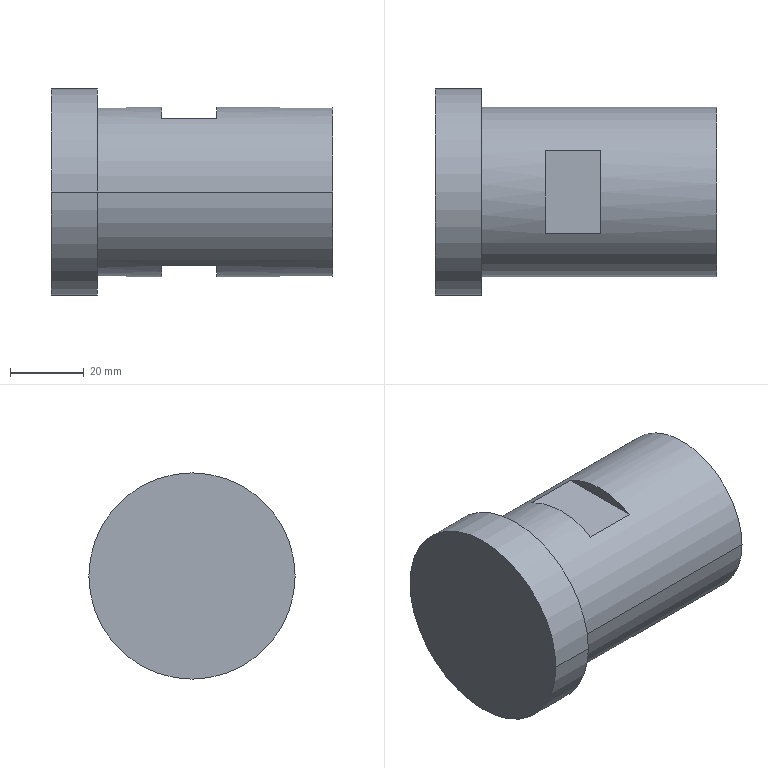Part | STEP file | DAU NOI BUA GIUA | 1 solid | 19 faces | box 76.5 x 56 x 56 mm | volume 107628 mm3 | plane 11 | cylinder 8 | commonest cylinder face diameters 33 x2 36 x2 46 x2 56 x2
STEP:
#1=CARTESIAN_POINT('',(0.,0.,0.));
#2=DIRECTION('',(0.,0.,1.));
#3=DIRECTION('',(1.,0.,0.));
#4=AXIS2_PLACEMENT_3D('',#1,#2,#3);
#5=CARTESIAN_POINT('',(45.,11.358,20.));
#6=VERTEX_POINT('',#5);
#7=CARTESIAN_POINT('',(45.,-11.358,20.));
#8=VERTEX_POINT('',#7);
#9=CARTESIAN_POINT('',(45.,0.,0.));
#10=DIRECTION('',(1.,0.,0.));
#11=DIRECTION('',(0.,1.,0.));
#12=AXIS2_PLACEMENT_3D('',#9,#10,#11);
#13=CIRCLE('',#12,23.);
#14=CARTESIAN_POINT('',(47.5,0.,0.));
#15=DIRECTION('',(1.,0.,0.));
#16=DIRECTION('',(0.,1.,0.));
#17=AXIS2_PLACEMENT_3D('',#14,#15,#16);
#18=CYLINDRICAL_SURFACE('',#17,23.);
#19=CARTESIAN_POINT('',(0.,-2.5));
#20=DIRECTION('',(1.,0.));
#21=VECTOR('',#20,1.);
#22=LINE('',#19,#21);
#23=(GEOMETRIC_REPRESENTATION_CONTEXT(2)PARAMETRIC_REPRESENTATION_CONTEXT()REPRESENTATION_CONTEXT('',''));
#24=DEFINITIONAL_REPRESENTATION('',(#22),#23);
#25=PCURVE('',#18,#24);
#26=CARTESIAN_POINT('',(45.,0.,20.));
#27=DIRECTION('',(1.,0.,0.));
#28=DIRECTION('',(0.,0.,-1.));
#29=AXIS2_PLACEMENT_3D('',#26,#27,#28);
#30=PLANE('',#29);
#31=CARTESIAN_POINT('',(20.,0.));
#32=DIRECTION('',(0.,1.));
#33=AXIS2_PLACEMENT_2D('',#31,#32);
#34=CIRCLE('',#33,23.);
#35=(GEOMETRIC_REPRESENTATION_CONTEXT(2)PARAMETRIC_REPRESENTATION_CONTEXT()REPRESENTATION_CONTEXT('',''));
#36=DEFINITIONAL_REPRESENTATION('',(#34),#35);
#37=PCURVE('',#30,#36);
#38=SURFACE_CURVE('',#13,(#25,#37),.PCURVE_S1.);
#39=EDGE_CURVE('',#6,#8,#38,.T.);
#40=ORIENTED_EDGE('',*,*,#39,.T.);
#41=CARTESIAN_POINT('',(30.,-11.358,20.));
#42=VERTEX_POINT('',#41);
#43=CARTESIAN_POINT('',(47.5,-11.358,20.));
#44=DIRECTION('',(-1.,0.,0.));
#45=VECTOR('',#44,1.);
#46=LINE('',#43,#45);
#47=CARTESIAN_POINT('',(2.087,0.));
#48=DIRECTION('',(0.,-1.));
#49=VECTOR('',#48,1.);
#50=LINE('',#47,#49);
#51=(GEOMETRIC_REPRESENTATION_CONTEXT(2)PARAMETRIC_REPRESENTATION_CONTEXT()REPRESENTATION_CONTEXT('',''));
#52=DEFINITIONAL_REPRESENTATION('',(#50),#51);
#53=PCURVE('',#18,#52);
#54=CARTESIAN_POINT('',(30.,0.,20.));
#55=DIRECTION('',(0.,0.,-1.));
#56=DIRECTION('',(-1.,0.,0.));
#57=AXIS2_PLACEMENT_3D('',#54,#55,#56);
#58=PLANE('',#57);
#59=CARTESIAN_POINT('',(-17.5,-11.358));
#60=DIRECTION('',(1.,0.));
#61=VECTOR('',#60,1.);
#62=LINE('',#59,#61);
#63=(GEOMETRIC_REPRESENTATION_CONTEXT(2)PARAMETRIC_REPRESENTATION_CONTEXT()REPRESENTATION_CONTEXT('',''));
#64=DEFINITIONAL_REPRESENTATION('',(#62),#63);
#65=PCURVE('',#58,#64);
#66=SURFACE_CURVE('',#46,(#53,#65),.PCURVE_S1.);
#67=EDGE_CURVE('',#8,#42,#66,.T.);
#68=ORIENTED_EDGE('',*,*,#67,.T.);
#69=CARTESIAN_POINT('',(30.,11.358,20.));
#70=VERTEX_POINT('',#69);
#71=CARTESIAN_POINT('',(30.,0.,0.));
#72=DIRECTION('',(-1.,0.,0.));
#73=DIRECTION('',(0.,1.,0.));
#74=AXIS2_PLACEMENT_3D('',#71,#72,#73);
#75=CIRCLE('',#74,23.);
#76=CARTESIAN_POINT('',(6.283,-17.5));
#77=DIRECTION('',(-1.,0.));
#78=VECTOR('',#77,1.);
#79=LINE('',#76,#78);
#80=(GEOMETRIC_REPRESENTATION_CONTEXT(2)PARAMETRIC_REPRESENTATION_CONTEXT()REPRESENTATION_CONTEXT('',''));
#81=DEFINITIONAL_REPRESENTATION('',(#79),#80);
#82=PCURVE('',#18,#81);
#83=CARTESIAN_POINT('',(30.,0.,30.));
#84=DIRECTION('',(-1.,0.,0.));
#85=DIRECTION('',(0.,0.,1.));
#86=AXIS2_PLACEMENT_3D('',#83,#84,#85);
#87=PLANE('',#86);
#88=CARTESIAN_POINT('',(-30.,0.));
#89=DIRECTION('',(0.,1.));
#90=AXIS2_PLACEMENT_2D('',#88,#89);
#91=CIRCLE('',#90,23.);
#92=(GEOMETRIC_REPRESENTATION_CONTEXT(2)PARAMETRIC_REPRESENTATION_CONTEXT()REPRESENTATION_CONTEXT('',''));
#93=DEFINITIONAL_REPRESENTATION('',(#91),#92);
#94=PCURVE('',#87,#93);
#95=SURFACE_CURVE('',#75,(#82,#94),.PCURVE_S1.);
#96=EDGE_CURVE('',#42,#70,#95,.T.);
#97=ORIENTED_EDGE('',*,*,#96,.T.);
#98=CARTESIAN_POINT('',(47.5,11.358,20.));
#99=DIRECTION('',(1.,0.,0.));
#100=VECTOR('',#99,1.);
#101=LINE('',#98,#100);
#102=CARTESIAN_POINT('',(1.054,0.));
#103=DIRECTION('',(0.,1.));
#104=VECTOR('',#103,1.);
#105=LINE('',#102,#104);
#106=(GEOMETRIC_REPRESENTATION_CONTEXT(2)PARAMETRIC_REPRESENTATION_CONTEXT()REPRESENTATION_CONTEXT('',''));
#107=DEFINITIONAL_REPRESENTATION('',(#105),#106);
#108=PCURVE('',#18,#107);
#109=CARTESIAN_POINT('',(-17.5,11.358));
#110=DIRECTION('',(-1.,0.));
#111=VECTOR('',#110,1.);
#112=LINE('',#109,#111);
#113=(GEOMETRIC_REPRESENTATION_CONTEXT(2)PARAMETRIC_REPRESENTATION_CONTEXT()REPRESENTATION_CONTEXT('',''));
#114=DEFINITIONAL_REPRESENTATION('',(#112),#113);
#115=PCURVE('',#58,#114);
#116=SURFACE_CURVE('',#101,(#108,#115),.PCURVE_S1.);
#117=EDGE_CURVE('',#70,#6,#116,.T.);
#118=ORIENTED_EDGE('',*,*,#117,.T.);
#119=EDGE_LOOP('',(#40,#68,#97,#118));
#120=FACE_BOUND('',#119,.T.);
#121=CARTESIAN_POINT('',(12.5,23.,0.));
#122=VERTEX_POINT('',#121);
#123=CARTESIAN_POINT('',(12.5,-23.,0.));
#124=VERTEX_POINT('',#123);
#125=CARTESIAN_POINT('',(12.5,0.,0.));
#126=DIRECTION('',(1.,0.,0.));
#127=DIRECTION('',(0.,1.,0.));
#128=AXIS2_PLACEMENT_3D('',#125,#126,#127);
#129=CIRCLE('',#128,23.);
#130=CARTESIAN_POINT('',(0.,-35.));
#131=DIRECTION('',(1.,0.));
#132=VECTOR('',#131,1.);
#133=LINE('',#130,#132);
#134=(GEOMETRIC_REPRESENTATION_CONTEXT(2)PARAMETRIC_REPRESENTATION_CONTEXT()REPRESENTATION_CONTEXT('',''));
#135=DEFINITIONAL_REPRESENTATION('',(#133),#134);
#136=PCURVE('',#18,#135);
#137=CARTESIAN_POINT('',(12.5,25.5,0.));
#138=DIRECTION('',(1.,0.,0.));
#139=DIRECTION('',(0.,0.,-1.));
#140=AXIS2_PLACEMENT_3D('',#137,#138,#139);
#141=PLANE('',#140);
#142=CARTESIAN_POINT('',(0.,-25.5));
#143=DIRECTION('',(0.,1.));
#144=AXIS2_PLACEMENT_2D('',#142,#143);
#145=CIRCLE('',#144,23.);
#146=(GEOMETRIC_REPRESENTATION_CONTEXT(2)PARAMETRIC_REPRESENTATION_CONTEXT()REPRESENTATION_CONTEXT('',''));
#147=DEFINITIONAL_REPRESENTATION('',(#145),#146);
#148=PCURVE('',#141,#147);
#149=SURFACE_CURVE('',#129,(#136,#148),.PCURVE_S1.);
#150=EDGE_CURVE('',#122,#124,#149,.T.);
#151=ORIENTED_EDGE('',*,*,#150,.T.);
#152=CARTESIAN_POINT('',(76.5,-23.,0.));
#153=VERTEX_POINT('',#152);
#154=CARTESIAN_POINT('',(47.5,-23.,0.));
#155=DIRECTION('',(1.,0.,0.));
#156=VECTOR('',#155,1.);
#157=LINE('',#154,#156);
#158=CARTESIAN_POINT('',(3.142,0.));
#159=DIRECTION('',(0.,1.));
#160=VECTOR('',#159,1.);
#161=LINE('',#158,#160);
#162=(GEOMETRIC_REPRESENTATION_CONTEXT(2)PARAMETRIC_REPRESENTATION_CONTEXT()REPRESENTATION_CONTEXT('',''));
#163=DEFINITIONAL_REPRESENTATION('',(#161),#162);
#164=PCURVE('',#18,#163);
#165=CARTESIAN_POINT('',(47.5,0.,0.));
#166=DIRECTION('',(1.,0.,0.));
#167=DIRECTION('',(0.,1.,0.));
#168=AXIS2_PLACEMENT_3D('',#165,#166,#167);
#169=CYLINDRICAL_SURFACE('',#168,23.);
#170=CARTESIAN_POINT('',(3.142,0.));
#171=DIRECTION('',(0.,1.));
#172=VECTOR('',#171,1.);
#173=LINE('',#170,#172);
#174=(GEOMETRIC_REPRESENTATION_CONTEXT(2)PARAMETRIC_REPRESENTATION_CONTEXT()REPRESENTATION_CONTEXT('',''));
#175=DEFINITIONAL_REPRESENTATION('',(#173),#174);
#176=PCURVE('',#169,#175);
#177=SURFACE_CURVE('',#157,(#164,#176),.PCURVE_S1.);
#178=EDGE_CURVE('',#124,#153,#177,.T.);
#179=ORIENTED_EDGE('',*,*,#178,.T.);
#180=CARTESIAN_POINT('',(76.5,23.,0.));
#181=VERTEX_POINT('',#180);
#182=CARTESIAN_POINT('',(76.5,0.,0.));
#183=DIRECTION('',(-1.,0.,0.));
#184=DIRECTION('',(0.,1.,0.));
#185=AXIS2_PLACEMENT_3D('',#182,#183,#184);
#186=CIRCLE('',#185,23.);
#187=CARTESIAN_POINT('',(6.283,29.));
#188=DIRECTION('',(-1.,0.));
#189=VECTOR('',#188,1.);
#190=LINE('',#187,#189);
#191=(GEOMETRIC_REPRESENTATION_CONTEXT(2)PARAMETRIC_REPRESENTATION_CONTEXT()REPRESENTATION_CONTEXT('',''));
#192=DEFINITIONAL_REPRESENTATION('',(#190),#191);
#193=PCURVE('',#18,#192);
#194=CARTESIAN_POINT('',(76.5,0.,0.));
#195=DIRECTION('',(-1.,0.,0.));
#196=DIRECTION('',(0.,0.,1.));
#197=AXIS2_PLACEMENT_3D('',#194,#195,#196);
#198=PLANE('',#197);
#199=CARTESIAN_POINT('',(0.,0.));
#200=DIRECTION('',(0.,1.));
#201=AXIS2_PLACEMENT_2D('',#199,#200);
#202=CIRCLE('',#201,23.);
#203=(GEOMETRIC_REPRESENTATION_CONTEXT(2)PARAMETRIC_REPRESENTATION_CONTEXT()REPRESENTATION_CONTEXT('',''));
#204=DEFINITIONAL_REPRESENTATION('',(#202),#203);
#205=PCURVE('',#198,#204);
#206=SURFACE_CURVE('',#186,(#193,#205),.PCURVE_S1.);
#207=EDGE_CURVE('',#153,#181,#206,.T.);
#208=ORIENTED_EDGE('',*,*,#207,.T.);
#209=CARTESIAN_POINT('',(47.5,23.,0.));
#210=DIRECTION('',(1.,0.,0.));
#211=VECTOR('',#210,1.);
#212=LINE('',#209,#211);
#213=CARTESIAN_POINT('',(0.,0.));
#214=DIRECTION('',(0.,1.));
#215=VECTOR('',#214,1.);
#216=LINE('',#213,#215);
#217=(GEOMETRIC_REPRESENTATION_CONTEXT(2)PARAMETRIC_REPRESENTATION_CONTEXT()REPRESENTATION_CONTEXT('',''));
#218=DEFINITIONAL_REPRESENTATION('',(#216),#217);
#219=PCURVE('',#18,#218);
#220=CARTESIAN_POINT('',(6.283,0.));
#221=DIRECTION('',(0.,1.));
#222=VECTOR('',#221,1.);
#223=LINE('',#220,#222);
#224=(GEOMETRIC_REPRESENTATION_CONTEXT(2)PARAMETRIC_REPRESENTATION_CONTEXT()REPRESENTATION_CONTEXT('',''));
#225=DEFINITIONAL_REPRESENTATION('',(#223),#224);
#226=PCURVE('',#169,#225);
#227=SURFACE_CURVE('',#212,(#219,#226),.PCURVE_S1.);
#228=EDGE_CURVE('',#122,#181,#227,.T.);
#229=ORIENTED_EDGE('',*,*,#228,.F.);
#230=EDGE_LOOP('',(#151,#179,#208,#229));
#231=FACE_BOUND('',#230,.T.);
#232=ADVANCED_FACE('',(#120,#231),#18,.T.);
#233=CARTESIAN_POINT('',(0.,28.,0.));
#234=VERTEX_POINT('',#233);
#235=CARTESIAN_POINT('',(0.,-28.,0.));
#236=VERTEX_POINT('',#235);
#237=CARTESIAN_POINT('',(0.,0.,0.));
#238=DIRECTION('',(1.,0.,0.));
#239=DIRECTION('',(0.,1.,0.));
#240=AXIS2_PLACEMENT_3D('',#237,#238,#239);
#241=CIRCLE('',#240,28.);
#242=CARTESIAN_POINT('',(6.25,0.,0.));
#243=DIRECTION('',(1.,0.,0.));
#244=DIRECTION('',(0.,1.,0.));
#245=AXIS2_PLACEMENT_3D('',#242,#243,#244);
#246=CYLINDRICAL_SURFACE('',#245,28.);
#247=CARTESIAN_POINT('',(0.,-6.25));
#248=DIRECTION('',(1.,0.));
#249=VECTOR('',#248,1.);
#250=LINE('',#247,#249);
#251=(GEOMETRIC_REPRESENTATION_CONTEXT(2)PARAMETRIC_REPRESENTATION_CONTEXT()REPRESENTATION_CONTEXT('',''));
#252=DEFINITIONAL_REPRESENTATION('',(#250),#251);
#253=PCURVE('',#246,#252);
#254=CARTESIAN_POINT('',(0.,14.,0.));
#255=DIRECTION('',(-1.,0.,0.));
#256=DIRECTION('',(0.,0.,1.));
#257=AXIS2_PLACEMENT_3D('',#254,#255,#256);
#258=PLANE('',#257);
#259=CARTESIAN_POINT('',(0.,14.));
#260=CARTESIAN_POINT('',(48.497,14.));
#261=CARTESIAN_POINT('',(24.249,-28.));
#262=CARTESIAN_POINT('',(0.,-70.));
#263=CARTESIAN_POINT('',(-24.249,-28.));
#264=CARTESIAN_POINT('',(-48.497,14.));
#265=CARTESIAN_POINT('',(0.,14.));
#266=(BOUNDED_CURVE()B_SPLINE_CURVE(2,(#259,#260,#261,#262,#263,#264,#265),.UNSPECIFIED.,.T.,.F.)B_SPLINE_CURVE_WITH_KNOTS((1,2,2,2,2,1),(-2.094,0.,2.094,4.189,6.283,8.378),.UNSPECIFIED.)CURVE()GEOMETRIC_REPRESENTATION_ITEM()RATIONAL_B_SPLINE_CURVE((1.,0.5,1.,0.5,1.,0.5,1.))REPRESENTATION_ITEM(''));
#267=(GEOMETRIC_REPRESENTATION_CONTEXT(2)PARAMETRIC_REPRESENTATION_CONTEXT()REPRESENTATION_CONTEXT('',''));
#268=DEFINITIONAL_REPRESENTATION('',(#266),#267);
#269=PCURVE('',#258,#268);
#270=SURFACE_CURVE('',#241,(#253,#269),.PCURVE_S1.);
#271=EDGE_CURVE('',#234,#236,#270,.T.);
#272=ORIENTED_EDGE('',*,*,#271,.T.);
#273=CARTESIAN_POINT('',(12.5,-28.,0.));
#274=VERTEX_POINT('',#273);
#275=CARTESIAN_POINT('',(6.25,-28.,0.));
#276=DIRECTION('',(1.,0.,0.));
#277=VECTOR('',#276,1.);
#278=LINE('',#275,#277);
#279=CARTESIAN_POINT('',(3.142,0.));
#280=DIRECTION('',(0.,1.));
#281=VECTOR('',#280,1.);
#282=LINE('',#279,#281);
#283=(GEOMETRIC_REPRESENTATION_CONTEXT(2)PARAMETRIC_REPRESENTATION_CONTEXT()REPRESENTATION_CONTEXT('',''));
#284=DEFINITIONAL_REPRESENTATION('',(#282),#283);
#285=PCURVE('',#246,#284);
#286=CARTESIAN_POINT('',(6.25,0.,0.));
#287=DIRECTION('',(1.,0.,0.));
#288=DIRECTION('',(0.,1.,0.));
#289=AXIS2_PLACEMENT_3D('',#286,#287,#288);
#290=CYLINDRICAL_SURFACE('',#289,28.);
#291=CARTESIAN_POINT('',(3.142,0.));
#292=DIRECTION('',(0.,1.));
#293=VECTOR('',#292,1.);
#294=LINE('',#291,#293);
#295=(GEOMETRIC_REPRESENTATION_CONTEXT(2)PARAMETRIC_REPRESENTATION_CONTEXT()REPRESENTATION_CONTEXT('',''));
#296=DEFINITIONAL_REPRESENTATION('',(#294),#295);
#297=PCURVE('',#290,#296);
#298=SURFACE_CURVE('',#278,(#285,#297),.PCURVE_S1.);
#299=EDGE_CURVE('',#236,#274,#298,.T.);
#300=ORIENTED_EDGE('',*,*,#299,.T.);
#301=CARTESIAN_POINT('',(12.5,28.,0.));
#302=VERTEX_POINT('',#301);
#303=CARTESIAN_POINT('',(12.5,0.,0.));
#304=DIRECTION('',(1.,0.,0.));
#305=DIRECTION('',(0.,1.,0.));
#306=AXIS2_PLACEMENT_3D('',#303,#304,#305);
#307=CIRCLE('',#306,28.);
#308=CARTESIAN_POINT('',(0.,6.25));
#309=DIRECTION('',(1.,0.));
#310=VECTOR('',#309,1.);
#311=LINE('',#308,#310);
#312=(GEOMETRIC_REPRESENTATION_CONTEXT(2)PARAMETRIC_REPRESENTATION_CONTEXT()REPRESENTATION_CONTEXT('',''));
#313=DEFINITIONAL_REPRESENTATION('',(#311),#312);
#314=PCURVE('',#246,#313);
#315=CARTESIAN_POINT('',(0.,-25.5));
#316=DIRECTION('',(0.,1.));
#317=AXIS2_PLACEMENT_2D('',#315,#316);
#318=CIRCLE('',#317,28.);
#319=(GEOMETRIC_REPRESENTATION_CONTEXT(2)PARAMETRIC_REPRESENTATION_CONTEXT()REPRESENTATION_CONTEXT('',''));
#320=DEFINITIONAL_REPRESENTATION('',(#318),#319);
#321=PCURVE('',#141,#320);
#322=SURFACE_CURVE('',#307,(#314,#321),.PCURVE_S1.);
#323=EDGE_CURVE('',#302,#274,#322,.T.);
#324=ORIENTED_EDGE('',*,*,#323,.F.);
#325=CARTESIAN_POINT('',(6.25,28.,0.));
#326=DIRECTION('',(1.,0.,0.));
#327=VECTOR('',#326,1.);
#328=LINE('',#325,#327);
#329=CARTESIAN_POINT('',(0.,0.));
#330=DIRECTION('',(0.,1.));
#331=VECTOR('',#330,1.);
#332=LINE('',#329,#331);
#333=(GEOMETRIC_REPRESENTATION_CONTEXT(2)PARAMETRIC_REPRESENTATION_CONTEXT()REPRESENTATION_CONTEXT('',''));
#334=DEFINITIONAL_REPRESENTATION('',(#332),#333);
#335=PCURVE('',#246,#334);
#336=CARTESIAN_POINT('',(6.283,0.));
#337=DIRECTION('',(0.,1.));
#338=VECTOR('',#337,1.);
#339=LINE('',#336,#338);
#340=(GEOMETRIC_REPRESENTATION_CONTEXT(2)PARAMETRIC_REPRESENTATION_CONTEXT()REPRESENTATION_CONTEXT('',''));
#341=DEFINITIONAL_REPRESENTATION('',(#339),#340);
#342=PCURVE('',#290,#341);
#343=SURFACE_CURVE('',#328,(#335,#342),.PCURVE_S1.);
#344=EDGE_CURVE('',#234,#302,#343,.T.);
#345=ORIENTED_EDGE('',*,*,#344,.F.);
#346=EDGE_LOOP('',(#272,#300,#324,#345));
#347=FACE_BOUND('',#346,.T.);
#348=ADVANCED_FACE('',(#347),#246,.T.);
#349=CARTESIAN_POINT('',(55.5,16.5,0.));
#350=VERTEX_POINT('',#349);
#351=CARTESIAN_POINT('',(76.5,16.5,0.));
#352=VERTEX_POINT('',#351);
#353=CARTESIAN_POINT('',(69.5,16.5,0.));
#354=DIRECTION('',(1.,0.,0.));
#355=VECTOR('',#354,1.);
#356=LINE('',#353,#355);
#357=CARTESIAN_POINT('',(69.5,0.,0.));
#358=DIRECTION('',(1.,0.,0.));
#359=DIRECTION('',(0.,1.,0.));
#360=AXIS2_PLACEMENT_3D('',#357,#358,#359);
#361=CYLINDRICAL_SURFACE('',#360,16.5);
#362=CARTESIAN_POINT('',(6.283,0.));
#363=DIRECTION('',(0.,1.));
#364=VECTOR('',#363,1.);
#365=LINE('',#362,#364);
#366=(GEOMETRIC_REPRESENTATION_CONTEXT(2)PARAMETRIC_REPRESENTATION_CONTEXT()REPRESENTATION_CONTEXT('',''));
#367=DEFINITIONAL_REPRESENTATION('',(#365),#366);
#368=PCURVE('',#361,#367);
#369=CARTESIAN_POINT('',(69.5,0.,0.));
#370=DIRECTION('',(1.,0.,0.));
#371=DIRECTION('',(0.,1.,0.));
#372=AXIS2_PLACEMENT_3D('',#369,#370,#371);
#373=CYLINDRICAL_SURFACE('',#372,16.5);
#374=CARTESIAN_POINT('',(0.,0.));
#375=DIRECTION('',(0.,1.));
#376=VECTOR('',#375,1.);
#377=LINE('',#374,#376);
#378=(GEOMETRIC_REPRESENTATION_CONTEXT(2)PARAMETRIC_REPRESENTATION_CONTEXT()REPRESENTATION_CONTEXT('',''));
#379=DEFINITIONAL_REPRESENTATION('',(#377),#378);
#380=PCURVE('',#373,#379);
#381=SURFACE_CURVE('',#356,(#368,#380),.PCURVE_S1.);
#382=EDGE_CURVE('',#350,#352,#381,.T.);
#383=ORIENTED_EDGE('',*,*,#382,.T.);
#384=CARTESIAN_POINT('',(76.5,-16.5,0.));
#385=VERTEX_POINT('',#384);
#386=CARTESIAN_POINT('',(76.5,0.,0.));
#387=DIRECTION('',(1.,0.,0.));
#388=DIRECTION('',(0.,1.,0.));
#389=AXIS2_PLACEMENT_3D('',#386,#387,#388);
#390=CIRCLE('',#389,16.5);
#391=CARTESIAN_POINT('',(0.,7.));
#392=DIRECTION('',(1.,0.));
#393=VECTOR('',#392,1.);
#394=LINE('',#391,#393);
#395=(GEOMETRIC_REPRESENTATION_CONTEXT(2)PARAMETRIC_REPRESENTATION_CONTEXT()REPRESENTATION_CONTEXT('',''));
#396=DEFINITIONAL_REPRESENTATION('',(#394),#395);
#397=PCURVE('',#361,#396);
#398=CARTESIAN_POINT('',(0.,16.5));
#399=CARTESIAN_POINT('',(28.579,16.5));
#400=CARTESIAN_POINT('',(14.289,-8.25));
#401=CARTESIAN_POINT('',(0.,-33.));
#402=CARTESIAN_POINT('',(-14.289,-8.25));
#403=CARTESIAN_POINT('',(-28.579,16.5));
#404=CARTESIAN_POINT('',(0.,16.5));
#405=(BOUNDED_CURVE()B_SPLINE_CURVE(2,(#398,#399,#400,#401,#402,#403,#404),.UNSPECIFIED.,.T.,.F.)B_SPLINE_CURVE_WITH_KNOTS((1,2,2,2,2,1),(-2.094,0.,2.094,4.189,6.283,8.378),.UNSPECIFIED.)CURVE()GEOMETRIC_REPRESENTATION_ITEM()RATIONAL_B_SPLINE_CURVE((1.,0.5,1.,0.5,1.,0.5,1.))REPRESENTATION_ITEM(''));
#406=(GEOMETRIC_REPRESENTATION_CONTEXT(2)PARAMETRIC_REPRESENTATION_CONTEXT()REPRESENTATION_CONTEXT('',''));
#407=DEFINITIONAL_REPRESENTATION('',(#405),#406);
#408=PCURVE('',#198,#407);
#409=SURFACE_CURVE('',#390,(#397,#408),.PCURVE_S1.);
#410=EDGE_CURVE('',#385,#352,#409,.T.);
#411=ORIENTED_EDGE('',*,*,#410,.F.);
#412=CARTESIAN_POINT('',(55.5,-16.5,0.));
#413=VERTEX_POINT('',#412);
#414=CARTESIAN_POINT('',(69.5,-16.5,0.));
#415=DIRECTION('',(1.,0.,0.));
#416=VECTOR('',#415,1.);
#417=LINE('',#414,#416);
#418=CARTESIAN_POINT('',(3.142,0.));
#419=DIRECTION('',(0.,1.));
#420=VECTOR('',#419,1.);
#421=LINE('',#418,#420);
#422=(GEOMETRIC_REPRESENTATION_CONTEXT(2)PARAMETRIC_REPRESENTATION_CONTEXT()REPRESENTATION_CONTEXT('',''));
#423=DEFINITIONAL_REPRESENTATION('',(#421),#422);
#424=PCURVE('',#361,#423);
#425=CARTESIAN_POINT('',(3.142,0.));
#426=DIRECTION('',(0.,1.));
#427=VECTOR('',#426,1.);
#428=LINE('',#425,#427);
#429=(GEOMETRIC_REPRESENTATION_CONTEXT(2)PARAMETRIC_REPRESENTATION_CONTEXT()REPRESENTATION_CONTEXT('',''));
#430=DEFINITIONAL_REPRESENTATION('',(#428),#429);
#431=PCURVE('',#373,#430);
#432=SURFACE_CURVE('',#417,(#424,#431),.PCURVE_S1.);
#433=EDGE_CURVE('',#413,#385,#432,.T.);
#434=ORIENTED_EDGE('',*,*,#433,.F.);
#435=CARTESIAN_POINT('',(55.5,0.,0.));
#436=DIRECTION('',(1.,0.,0.));
#437=DIRECTION('',(0.,1.,0.));
#438=AXIS2_PLACEMENT_3D('',#435,#436,#437);
#439=CIRCLE('',#438,16.5);
#440=CARTESIAN_POINT('',(0.,-14.));
#441=DIRECTION('',(1.,0.));
#442=VECTOR('',#441,1.);
#443=LINE('',#440,#442);
#444=(GEOMETRIC_REPRESENTATION_CONTEXT(2)PARAMETRIC_REPRESENTATION_CONTEXT()REPRESENTATION_CONTEXT('',''));
#445=DEFINITIONAL_REPRESENTATION('',(#443),#444);
#446=PCURVE('',#361,#445);
#447=CARTESIAN_POINT('',(55.5,17.25,0.));
#448=DIRECTION('',(-1.,0.,0.));
#449=DIRECTION('',(0.,0.,1.));
#450=AXIS2_PLACEMENT_3D('',#447,#448,#449);
#451=PLANE('',#450);
#452=CARTESIAN_POINT('',(0.,-0.75));
#453=CARTESIAN_POINT('',(28.579,-0.75));
#454=CARTESIAN_POINT('',(14.289,-25.5));
#455=CARTESIAN_POINT('',(0.,-50.25));
#456=CARTESIAN_POINT('',(-14.289,-25.5));
#457=CARTESIAN_POINT('',(-28.579,-0.75));
#458=CARTESIAN_POINT('',(0.,-0.75));
#459=(BOUNDED_CURVE()B_SPLINE_CURVE(2,(#452,#453,#454,#455,#456,#457,#458),.UNSPECIFIED.,.T.,.F.)B_SPLINE_CURVE_WITH_KNOTS((1,2,2,2,2,1),(-2.094,0.,2.094,4.189,6.283,8.378),.UNSPECIFIED.)CURVE()GEOMETRIC_REPRESENTATION_ITEM()RATIONAL_B_SPLINE_CURVE((1.,0.5,1.,0.5,1.,0.5,1.))REPRESENTATION_ITEM(''));
#460=(GEOMETRIC_REPRESENTATION_CONTEXT(2)PARAMETRIC_REPRESENTATION_CONTEXT()REPRESENTATION_CONTEXT('',''));
#461=DEFINITIONAL_REPRESENTATION('',(#459),#460);
#462=PCURVE('',#451,#461);
#463=SURFACE_CURVE('',#439,(#446,#462),.PCURVE_S1.);
#464=EDGE_CURVE('',#413,#350,#463,.T.);
#465=ORIENTED_EDGE('',*,*,#464,.T.);
#466=EDGE_LOOP('',(#383,#411,#434,#465));
#467=FACE_BOUND('',#466,.F.);
#468=ADVANCED_FACE('',(#467),#361,.F.);
#469=CARTESIAN_POINT('',(45.5,18.,0.));
#470=VERTEX_POINT('',#469);
#471=CARTESIAN_POINT('',(55.5,18.,0.));
#472=VERTEX_POINT('',#471);
#473=CARTESIAN_POINT('',(50.5,18.,0.));
#474=DIRECTION('',(1.,0.,0.));
#475=VECTOR('',#474,1.);
#476=LINE('',#473,#475);
#477=CARTESIAN_POINT('',(50.5,0.,0.));
#478=DIRECTION('',(1.,0.,0.));
#479=DIRECTION('',(0.,1.,0.));
#480=AXIS2_PLACEMENT_3D('',#477,#478,#479);
#481=CYLINDRICAL_SURFACE('',#480,18.);
#482=CARTESIAN_POINT('',(6.283,0.));
#483=DIRECTION('',(0.,1.));
#484=VECTOR('',#483,1.);
#485=LINE('',#482,#484);
#486=(GEOMETRIC_REPRESENTATION_CONTEXT(2)PARAMETRIC_REPRESENTATION_CONTEXT()REPRESENTATION_CONTEXT('',''));
#487=DEFINITIONAL_REPRESENTATION('',(#485),#486);
#488=PCURVE('',#481,#487);
#489=CARTESIAN_POINT('',(50.5,0.,0.));
#490=DIRECTION('',(1.,0.,0.));
#491=DIRECTION('',(0.,1.,0.));
#492=AXIS2_PLACEMENT_3D('',#489,#490,#491);
#493=CYLINDRICAL_SURFACE('',#492,18.);
#494=CARTESIAN_POINT('',(0.,0.));
#495=DIRECTION('',(0.,1.));
#496=VECTOR('',#495,1.);
#497=LINE('',#494,#496);
#498=(GEOMETRIC_REPRESENTATION_CONTEXT(2)PARAMETRIC_REPRESENTATION_CONTEXT()REPRESENTATION_CONTEXT('',''));
#499=DEFINITIONAL_REPRESENTATION('',(#497),#498);
#500=PCURVE('',#493,#499);
#501=SURFACE_CURVE('',#476,(#488,#500),.PCURVE_S1.);
#502=EDGE_CURVE('',#470,#472,#501,.T.);
#503=ORIENTED_EDGE('',*,*,#502,.T.);
#504=CARTESIAN_POINT('',(55.5,-18.,0.));
#505=VERTEX_POINT('',#504);
#506=CARTESIAN_POINT('',(55.5,0.,0.));
#507=DIRECTION('',(-1.,0.,0.));
#508=DIRECTION('',(0.,1.,0.));
#509=AXIS2_PLACEMENT_3D('',#506,#507,#508);
#510=CIRCLE('',#509,18.);
#511=CARTESIAN_POINT('',(6.283,5.));
#512=DIRECTION('',(-1.,0.));
#513=VECTOR('',#512,1.);
#514=LINE('',#511,#513);
#515=(GEOMETRIC_REPRESENTATION_CONTEXT(2)PARAMETRIC_REPRESENTATION_CONTEXT()REPRESENTATION_CONTEXT('',''));
#516=DEFINITIONAL_REPRESENTATION('',(#514),#515);
#517=PCURVE('',#481,#516);
#518=CARTESIAN_POINT('',(0.,-17.25));
#519=DIRECTION('',(0.,1.));
#520=AXIS2_PLACEMENT_2D('',#518,#519);
#521=CIRCLE('',#520,18.);
#522=(GEOMETRIC_REPRESENTATION_CONTEXT(2)PARAMETRIC_REPRESENTATION_CONTEXT()REPRESENTATION_CONTEXT('',''));
#523=DEFINITIONAL_REPRESENTATION('',(#521),#522);
#524=PCURVE('',#451,#523);
#525=SURFACE_CURVE('',#510,(#517,#524),.PCURVE_S1.);
#526=EDGE_CURVE('',#472,#505,#525,.T.);
#527=ORIENTED_EDGE('',*,*,#526,.T.);
#528=CARTESIAN_POINT('',(45.5,-18.,0.));
#529=VERTEX_POINT('',#528);
#530=CARTESIAN_POINT('',(50.5,-18.,0.));
#531=DIRECTION('',(1.,0.,0.));
#532=VECTOR('',#531,1.);
#533=LINE('',#530,#532);
#534=CARTESIAN_POINT('',(3.142,0.));
#535=DIRECTION('',(0.,1.));
#536=VECTOR('',#535,1.);
#537=LINE('',#534,#536);
#538=(GEOMETRIC_REPRESENTATION_CONTEXT(2)PARAMETRIC_REPRESENTATION_CONTEXT()REPRESENTATION_CONTEXT('',''));
#539=DEFINITIONAL_REPRESENTATION('',(#537),#538);
#540=PCURVE('',#481,#539);
#541=CARTESIAN_POINT('',(3.142,0.));
#542=DIRECTION('',(0.,1.));
#543=VECTOR('',#542,1.);
#544=LINE('',#541,#543);
#545=(GEOMETRIC_REPRESENTATION_CONTEXT(2)PARAMETRIC_REPRESENTATION_CONTEXT()REPRESENTATION_CONTEXT('',''));
#546=DEFINITIONAL_REPRESENTATION('',(#544),#545);
#547=PCURVE('',#493,#546);
#548=SURFACE_CURVE('',#533,(#540,#547),.PCURVE_S1.);
#549=EDGE_CURVE('',#529,#505,#548,.T.);
#550=ORIENTED_EDGE('',*,*,#549,.F.);
#551=CARTESIAN_POINT('',(45.5,0.,0.));
#552=DIRECTION('',(1.,0.,0.));
#553=DIRECTION('',(0.,1.,0.));
#554=AXIS2_PLACEMENT_3D('',#551,#552,#553);
#555=CIRCLE('',#554,18.);
#556=CARTESIAN_POINT('',(0.,-5.));
#557=DIRECTION('',(1.,0.));
#558=VECTOR('',#557,1.);
#559=LINE('',#556,#558);
#560=(GEOMETRIC_REPRESENTATION_CONTEXT(2)PARAMETRIC_REPRESENTATION_CONTEXT()REPRESENTATION_CONTEXT('',''));
#561=DEFINITIONAL_REPRESENTATION('',(#559),#560);
#562=PCURVE('',#481,#561);
#563=CARTESIAN_POINT('',(45.5,8.75,0.));
#564=DIRECTION('',(1.,0.,0.));
#565=DIRECTION('',(0.,0.,-1.));
#566=AXIS2_PLACEMENT_3D('',#563,#564,#565);
#567=PLANE('',#566);
#568=CARTESIAN_POINT('',(0.,-8.75));
#569=DIRECTION('',(0.,1.));
#570=AXIS2_PLACEMENT_2D('',#568,#569);
#571=CIRCLE('',#570,18.);
#572=(GEOMETRIC_REPRESENTATION_CONTEXT(2)PARAMETRIC_REPRESENTATION_CONTEXT()REPRESENTATION_CONTEXT('',''));
#573=DEFINITIONAL_REPRESENTATION('',(#571),#572);
#574=PCURVE('',#567,#573);
#575=SURFACE_CURVE('',#555,(#562,#574),.PCURVE_S1.);
#576=EDGE_CURVE('',#529,#470,#575,.T.);
#577=ORIENTED_EDGE('',*,*,#576,.T.);
#578=EDGE_LOOP('',(#503,#527,#550,#577));
#579=FACE_BOUND('',#578,.F.);
#580=ADVANCED_FACE('',(#579),#481,.F.);
#581=ORIENTED_EDGE('',*,*,#178,.F.);
#582=CARTESIAN_POINT('',(12.5,0.,0.));
#583=DIRECTION('',(1.,0.,0.));
#584=DIRECTION('',(0.,1.,0.));
#585=AXIS2_PLACEMENT_3D('',#582,#583,#584);
#586=CIRCLE('',#585,23.);
#587=CARTESIAN_POINT('',(0.,-35.));
#588=DIRECTION('',(1.,0.));
#589=VECTOR('',#588,1.);
#590=LINE('',#587,#589);
#591=(GEOMETRIC_REPRESENTATION_CONTEXT(2)PARAMETRIC_REPRESENTATION_CONTEXT()REPRESENTATION_CONTEXT('',''));
#592=DEFINITIONAL_REPRESENTATION('',(#590),#591);
#593=PCURVE('',#169,#592);
#594=CARTESIAN_POINT('',(0.,-25.5));
#595=DIRECTION('',(0.,1.));
#596=AXIS2_PLACEMENT_2D('',#594,#595);
#597=CIRCLE('',#596,23.);
#598=(GEOMETRIC_REPRESENTATION_CONTEXT(2)PARAMETRIC_REPRESENTATION_CONTEXT()REPRESENTATION_CONTEXT('',''));
#599=DEFINITIONAL_REPRESENTATION('',(#597),#598);
#600=PCURVE('',#141,#599);
#601=SURFACE_CURVE('',#586,(#593,#600),.PCURVE_S1.);
#602=EDGE_CURVE('',#124,#122,#601,.T.);
#603=ORIENTED_EDGE('',*,*,#602,.T.);
#604=ORIENTED_EDGE('',*,*,#228,.T.);
#605=CARTESIAN_POINT('',(76.5,0.,0.));
#606=DIRECTION('',(-1.,0.,0.));
#607=DIRECTION('',(0.,1.,0.));
#608=AXIS2_PLACEMENT_3D('',#605,#606,#607);
#609=CIRCLE('',#608,23.);
#610=CARTESIAN_POINT('',(6.283,29.));
#611=DIRECTION('',(-1.,0.));
#612=VECTOR('',#611,1.);
#613=LINE('',#610,#612);
#614=(GEOMETRIC_REPRESENTATION_CONTEXT(2)PARAMETRIC_REPRESENTATION_CONTEXT()REPRESENTATION_CONTEXT('',''));
#615=DEFINITIONAL_REPRESENTATION('',(#613),#614);
#616=PCURVE('',#169,#615);
#617=CARTESIAN_POINT('',(0.,0.));
#618=DIRECTION('',(0.,1.));
#619=AXIS2_PLACEMENT_2D('',#617,#618);
#620=CIRCLE('',#619,23.);
#621=(GEOMETRIC_REPRESENTATION_CONTEXT(2)PARAMETRIC_REPRESENTATION_CONTEXT()REPRESENTATION_CONTEXT('',''));
#622=DEFINITIONAL_REPRESENTATION('',(#620),#621);
#623=PCURVE('',#198,#622);
#624=SURFACE_CURVE('',#609,(#616,#623),.PCURVE_S1.);
#625=EDGE_CURVE('',#181,#153,#624,.T.);
#626=ORIENTED_EDGE('',*,*,#625,.T.);
#627=EDGE_LOOP('',(#581,#603,#604,#626));
#628=FACE_BOUND('',#627,.T.);
#629=CARTESIAN_POINT('',(30.,11.358,-20.));
#630=VERTEX_POINT('',#629);
#631=CARTESIAN_POINT('',(30.,-11.358,-20.));
#632=VERTEX_POINT('',#631);
#633=CARTESIAN_POINT('',(30.,0.,0.));
#634=DIRECTION('',(-1.,0.,0.));
#635=DIRECTION('',(0.,1.,0.));
#636=AXIS2_PLACEMENT_3D('',#633,#634,#635);
#637=CIRCLE('',#636,23.);
#638=CARTESIAN_POINT('',(6.283,-17.5));
#639=DIRECTION('',(-1.,0.));
#640=VECTOR('',#639,1.);
#641=LINE('',#638,#640);
#642=(GEOMETRIC_REPRESENTATION_CONTEXT(2)PARAMETRIC_REPRESENTATION_CONTEXT()REPRESENTATION_CONTEXT('',''));
#643=DEFINITIONAL_REPRESENTATION('',(#641),#642);
#644=PCURVE('',#169,#643);
#645=CARTESIAN_POINT('',(30.,0.,-20.));
#646=DIRECTION('',(-1.,0.,0.));
#647=DIRECTION('',(0.,0.,1.));
#648=AXIS2_PLACEMENT_3D('',#645,#646,#647);
#649=PLANE('',#648);
#650=CARTESIAN_POINT('',(20.,0.));
#651=DIRECTION('',(0.,1.));
#652=AXIS2_PLACEMENT_2D('',#650,#651);
#653=CIRCLE('',#652,23.);
#654=(GEOMETRIC_REPRESENTATION_CONTEXT(2)PARAMETRIC_REPRESENTATION_CONTEXT()REPRESENTATION_CONTEXT('',''));
#655=DEFINITIONAL_REPRESENTATION('',(#653),#654);
#656=PCURVE('',#649,#655);
#657=SURFACE_CURVE('',#637,(#644,#656),.PCURVE_S1.);
#658=EDGE_CURVE('',#630,#632,#657,.T.);
#659=ORIENTED_EDGE('',*,*,#658,.T.);
#660=CARTESIAN_POINT('',(45.,-11.358,-20.));
#661=VERTEX_POINT('',#660);
#662=CARTESIAN_POINT('',(47.5,-11.358,-20.));
#663=DIRECTION('',(1.,0.,0.));
#664=VECTOR('',#663,1.);
#665=LINE('',#662,#664);
#666=CARTESIAN_POINT('',(4.196,0.));
#667=DIRECTION('',(0.,1.));
#668=VECTOR('',#667,1.);
#669=LINE('',#666,#668);
#670=(GEOMETRIC_REPRESENTATION_CONTEXT(2)PARAMETRIC_REPRESENTATION_CONTEXT()REPRESENTATION_CONTEXT('',''));
#671=DEFINITIONAL_REPRESENTATION('',(#669),#670);
#672=PCURVE('',#169,#671);
#673=CARTESIAN_POINT('',(45.,0.,-20.));
#674=DIRECTION('',(0.,0.,1.));
#675=DIRECTION('',(1.,0.,0.));
#676=AXIS2_PLACEMENT_3D('',#673,#674,#675);
#677=PLANE('',#676);
#678=CARTESIAN_POINT('',(2.5,-11.358));
#679=DIRECTION('',(1.,0.));
#680=VECTOR('',#679,1.);
#681=LINE('',#678,#680);
#682=(GEOMETRIC_REPRESENTATION_CONTEXT(2)PARAMETRIC_REPRESENTATION_CONTEXT()REPRESENTATION_CONTEXT('',''));
#683=DEFINITIONAL_REPRESENTATION('',(#681),#682);
#684=PCURVE('',#677,#683);
#685=SURFACE_CURVE('',#665,(#672,#684),.PCURVE_S1.);
#686=EDGE_CURVE('',#632,#661,#685,.T.);
#687=ORIENTED_EDGE('',*,*,#686,.T.);
#688=CARTESIAN_POINT('',(45.,11.358,-20.));
#689=VERTEX_POINT('',#688);
#690=CARTESIAN_POINT('',(45.,0.,0.));
#691=DIRECTION('',(1.,0.,0.));
#692=DIRECTION('',(0.,1.,0.));
#693=AXIS2_PLACEMENT_3D('',#690,#691,#692);
#694=CIRCLE('',#693,23.);
#695=CARTESIAN_POINT('',(0.,-2.5));
#696=DIRECTION('',(1.,0.));
#697=VECTOR('',#696,1.);
#698=LINE('',#695,#697);
#699=(GEOMETRIC_REPRESENTATION_CONTEXT(2)PARAMETRIC_REPRESENTATION_CONTEXT()REPRESENTATION_CONTEXT('',''));
#700=DEFINITIONAL_REPRESENTATION('',(#698),#699);
#701=PCURVE('',#169,#700);
#702=CARTESIAN_POINT('',(45.,0.,-30.));
#703=DIRECTION('',(1.,0.,0.));
#704=DIRECTION('',(0.,0.,-1.));
#705=AXIS2_PLACEMENT_3D('',#702,#703,#704);
#706=PLANE('',#705);
#707=CARTESIAN_POINT('',(-30.,0.));
#708=DIRECTION('',(0.,1.));
#709=AXIS2_PLACEMENT_2D('',#707,#708);
#710=CIRCLE('',#709,23.);
#711=(GEOMETRIC_REPRESENTATION_CONTEXT(2)PARAMETRIC_REPRESENTATION_CONTEXT()REPRESENTATION_CONTEXT('',''));
#712=DEFINITIONAL_REPRESENTATION('',(#710),#711);
#713=PCURVE('',#706,#712);
#714=SURFACE_CURVE('',#694,(#701,#713),.PCURVE_S1.);
#715=EDGE_CURVE('',#661,#689,#714,.T.);
#716=ORIENTED_EDGE('',*,*,#715,.T.);
#717=CARTESIAN_POINT('',(47.5,11.358,-20.));
#718=DIRECTION('',(-1.,0.,0.));
#719=VECTOR('',#718,1.);
#720=LINE('',#717,#719);
#721=CARTESIAN_POINT('',(5.229,0.));
#722=DIRECTION('',(0.,-1.));
#723=VECTOR('',#722,1.);
#724=LINE('',#721,#723);
#725=(GEOMETRIC_REPRESENTATION_CONTEXT(2)PARAMETRIC_REPRESENTATION_CONTEXT()REPRESENTATION_CONTEXT('',''));
#726=DEFINITIONAL_REPRESENTATION('',(#724),#725);
#727=PCURVE('',#169,#726);
#728=CARTESIAN_POINT('',(2.5,11.358));
#729=DIRECTION('',(-1.,0.));
#730=VECTOR('',#729,1.);
#731=LINE('',#728,#730);
#732=(GEOMETRIC_REPRESENTATION_CONTEXT(2)PARAMETRIC_REPRESENTATION_CONTEXT()REPRESENTATION_CONTEXT('',''));
#733=DEFINITIONAL_REPRESENTATION('',(#731),#732);
#734=PCURVE('',#677,#733);
#735=SURFACE_CURVE('',#720,(#727,#734),.PCURVE_S1.);
#736=EDGE_CURVE('',#689,#630,#735,.T.);
#737=ORIENTED_EDGE('',*,*,#736,.T.);
#738=EDGE_LOOP('',(#659,#687,#716,#737));
#739=FACE_BOUND('',#738,.T.);
#740=ADVANCED_FACE('',(#628,#739),#169,.T.);
#741=ORIENTED_EDGE('',*,*,#150,.F.);
#742=ORIENTED_EDGE('',*,*,#602,.F.);
#743=EDGE_LOOP('',(#741,#742));
#744=FACE_BOUND('',#743,.T.);
#745=ORIENTED_EDGE('',*,*,#323,.T.);
#746=CARTESIAN_POINT('',(12.5,0.,0.));
#747=DIRECTION('',(1.,0.,0.));
#748=DIRECTION('',(0.,1.,0.));
#749=AXIS2_PLACEMENT_3D('',#746,#747,#748);
#750=CIRCLE('',#749,28.);
#751=CARTESIAN_POINT('',(0.,-25.5));
#752=DIRECTION('',(0.,1.));
#753=AXIS2_PLACEMENT_2D('',#751,#752);
#754=CIRCLE('',#753,28.);
#755=(GEOMETRIC_REPRESENTATION_CONTEXT(2)PARAMETRIC_REPRESENTATION_CONTEXT()REPRESENTATION_CONTEXT('',''));
#756=DEFINITIONAL_REPRESENTATION('',(#754),#755);
#757=PCURVE('',#141,#756);
#758=CARTESIAN_POINT('',(0.,6.25));
#759=DIRECTION('',(1.,0.));
#760=VECTOR('',#759,1.);
#761=LINE('',#758,#760);
#762=(GEOMETRIC_REPRESENTATION_CONTEXT(2)PARAMETRIC_REPRESENTATION_CONTEXT()REPRESENTATION_CONTEXT('',''));
#763=DEFINITIONAL_REPRESENTATION('',(#761),#762);
#764=PCURVE('',#290,#763);
#765=SURFACE_CURVE('',#750,(#757,#764),.PCURVE_S1.);
#766=EDGE_CURVE('',#274,#302,#765,.T.);
#767=ORIENTED_EDGE('',*,*,#766,.T.);
#768=EDGE_LOOP('',(#745,#767));
#769=FACE_BOUND('',#768,.T.);
#770=ADVANCED_FACE('',(#744,#769),#141,.T.);
#771=CARTESIAN_POINT('',(30.,0.,20.));
#772=DIRECTION('',(0.,1.,0.));
#773=VECTOR('',#772,1.);
#774=LINE('',#771,#773);
#775=CARTESIAN_POINT('',(0.,0.));
#776=DIRECTION('',(0.,1.));
#777=VECTOR('',#776,1.);
#778=LINE('',#775,#777);
#779=(GEOMETRIC_REPRESENTATION_CONTEXT(2)PARAMETRIC_REPRESENTATION_CONTEXT()REPRESENTATION_CONTEXT('',''));
#780=DEFINITIONAL_REPRESENTATION('',(#778),#779);
#781=PCURVE('',#58,#780);
#782=CARTESIAN_POINT('',(-10.,0.));
#783=DIRECTION('',(0.,1.));
#784=VECTOR('',#783,1.);
#785=LINE('',#782,#784);
#786=(GEOMETRIC_REPRESENTATION_CONTEXT(2)PARAMETRIC_REPRESENTATION_CONTEXT()REPRESENTATION_CONTEXT('',''));
#787=DEFINITIONAL_REPRESENTATION('',(#785),#786);
#788=PCURVE('',#87,#787);
#789=SURFACE_CURVE('',#774,(#781,#788),.PCURVE_S1.);
#790=EDGE_CURVE('',#42,#70,#789,.T.);
#791=ORIENTED_EDGE('',*,*,#790,.F.);
#792=ORIENTED_EDGE('',*,*,#67,.F.);
#793=CARTESIAN_POINT('',(45.,0.,20.));
#794=DIRECTION('',(0.,-1.,0.));
#795=VECTOR('',#794,1.);
#796=LINE('',#793,#795);
#797=CARTESIAN_POINT('',(-15.,0.));
#798=DIRECTION('',(0.,-1.));
#799=VECTOR('',#798,1.);
#800=LINE('',#797,#799);
#801=(GEOMETRIC_REPRESENTATION_CONTEXT(2)PARAMETRIC_REPRESENTATION_CONTEXT()REPRESENTATION_CONTEXT('',''));
#802=DEFINITIONAL_REPRESENTATION('',(#800),#801);
#803=PCURVE('',#58,#802);
#804=CARTESIAN_POINT('',(0.,0.));
#805=DIRECTION('',(0.,-1.));
#806=VECTOR('',#805,1.);
#807=LINE('',#804,#806);
#808=(GEOMETRIC_REPRESENTATION_CONTEXT(2)PARAMETRIC_REPRESENTATION_CONTEXT()REPRESENTATION_CONTEXT('',''));
#809=DEFINITIONAL_REPRESENTATION('',(#807),#808);
#810=PCURVE('',#30,#809);
#811=SURFACE_CURVE('',#796,(#803,#810),.PCURVE_S1.);
#812=EDGE_CURVE('',#6,#8,#811,.T.);
#813=ORIENTED_EDGE('',*,*,#812,.F.);
#814=ORIENTED_EDGE('',*,*,#117,.F.);
#815=EDGE_LOOP('',(#791,#792,#813,#814));
#816=FACE_BOUND('',#815,.T.);
#817=ADVANCED_FACE('',(#816),#58,.F.);
#818=ORIENTED_EDGE('',*,*,#812,.T.);
#819=ORIENTED_EDGE('',*,*,#39,.F.);
#820=EDGE_LOOP('',(#818,#819));
#821=FACE_BOUND('',#820,.T.);
#822=ADVANCED_FACE('',(#821),#30,.F.);
#823=ORIENTED_EDGE('',*,*,#790,.T.);
#824=ORIENTED_EDGE('',*,*,#96,.F.);
#825=EDGE_LOOP('',(#823,#824));
#826=FACE_BOUND('',#825,.T.);
#827=ADVANCED_FACE('',(#826),#87,.F.);
#828=CARTESIAN_POINT('',(45.,0.,-20.));
#829=DIRECTION('',(0.,1.,0.));
#830=VECTOR('',#829,1.);
#831=LINE('',#828,#830);
#832=CARTESIAN_POINT('',(0.,0.));
#833=DIRECTION('',(0.,1.));
#834=VECTOR('',#833,1.);
#835=LINE('',#832,#834);
#836=(GEOMETRIC_REPRESENTATION_CONTEXT(2)PARAMETRIC_REPRESENTATION_CONTEXT()REPRESENTATION_CONTEXT('',''));
#837=DEFINITIONAL_REPRESENTATION('',(#835),#836);
#838=PCURVE('',#677,#837);
#839=CARTESIAN_POINT('',(-10.,0.));
#840=DIRECTION('',(0.,1.));
#841=VECTOR('',#840,1.);
#842=LINE('',#839,#841);
#843=(GEOMETRIC_REPRESENTATION_CONTEXT(2)PARAMETRIC_REPRESENTATION_CONTEXT()REPRESENTATION_CONTEXT('',''));
#844=DEFINITIONAL_REPRESENTATION('',(#842),#843);
#845=PCURVE('',#706,#844);
#846=SURFACE_CURVE('',#831,(#838,#845),.PCURVE_S1.);
#847=EDGE_CURVE('',#661,#689,#846,.T.);
#848=ORIENTED_EDGE('',*,*,#847,.F.);
#849=ORIENTED_EDGE('',*,*,#686,.F.);
#850=CARTESIAN_POINT('',(30.,0.,-20.));
#851=DIRECTION('',(0.,-1.,0.));
#852=VECTOR('',#851,1.);
#853=LINE('',#850,#852);
#854=CARTESIAN_POINT('',(-15.,0.));
#855=DIRECTION('',(0.,-1.));
#856=VECTOR('',#855,1.);
#857=LINE('',#854,#856);
#858=(GEOMETRIC_REPRESENTATION_CONTEXT(2)PARAMETRIC_REPRESENTATION_CONTEXT()REPRESENTATION_CONTEXT('',''));
#859=DEFINITIONAL_REPRESENTATION('',(#857),#858);
#860=PCURVE('',#677,#859);
#861=CARTESIAN_POINT('',(0.,0.));
#862=DIRECTION('',(0.,-1.));
#863=VECTOR('',#862,1.);
#864=LINE('',#861,#863);
#865=(GEOMETRIC_REPRESENTATION_CONTEXT(2)PARAMETRIC_REPRESENTATION_CONTEXT()REPRESENTATION_CONTEXT('',''));
#866=DEFINITIONAL_REPRESENTATION('',(#864),#865);
#867=PCURVE('',#649,#866);
#868=SURFACE_CURVE('',#853,(#860,#867),.PCURVE_S1.);
#869=EDGE_CURVE('',#630,#632,#868,.T.);
#870=ORIENTED_EDGE('',*,*,#869,.F.);
#871=ORIENTED_EDGE('',*,*,#736,.F.);
#872=EDGE_LOOP('',(#848,#849,#870,#871));
#873=FACE_BOUND('',#872,.T.);
#874=ADVANCED_FACE('',(#873),#677,.F.);
#875=ORIENTED_EDGE('',*,*,#869,.T.);
#876=ORIENTED_EDGE('',*,*,#658,.F.);
#877=EDGE_LOOP('',(#875,#876));
#878=FACE_BOUND('',#877,.T.);
#879=ADVANCED_FACE('',(#878),#649,.F.);
#880=ORIENTED_EDGE('',*,*,#847,.T.);
#881=ORIENTED_EDGE('',*,*,#715,.F.);
#882=EDGE_LOOP('',(#880,#881));
#883=FACE_BOUND('',#882,.T.);
#884=ADVANCED_FACE('',(#883),#706,.F.);
#885=CARTESIAN_POINT('',(76.5,0.,0.));
#886=DIRECTION('',(1.,0.,0.));
#887=DIRECTION('',(0.,1.,0.));
#888=AXIS2_PLACEMENT_3D('',#885,#886,#887);
#889=CIRCLE('',#888,16.5);
#890=CARTESIAN_POINT('',(0.,16.5));
#891=CARTESIAN_POINT('',(28.579,16.5));
#892=CARTESIAN_POINT('',(14.289,-8.25));
#893=CARTESIAN_POINT('',(0.,-33.));
#894=CARTESIAN_POINT('',(-14.289,-8.25));
#895=CARTESIAN_POINT('',(-28.579,16.5));
#896=CARTESIAN_POINT('',(0.,16.5));
#897=(BOUNDED_CURVE()B_SPLINE_CURVE(2,(#890,#891,#892,#893,#894,#895,#896),.UNSPECIFIED.,.T.,.F.)B_SPLINE_CURVE_WITH_KNOTS((1,2,2,2,2,1),(-2.094,0.,2.094,4.189,6.283,8.378),.UNSPECIFIED.)CURVE()GEOMETRIC_REPRESENTATION_ITEM()RATIONAL_B_SPLINE_CURVE((1.,0.5,1.,0.5,1.,0.5,1.))REPRESENTATION_ITEM(''));
#898=(GEOMETRIC_REPRESENTATION_CONTEXT(2)PARAMETRIC_REPRESENTATION_CONTEXT()REPRESENTATION_CONTEXT('',''));
#899=DEFINITIONAL_REPRESENTATION('',(#897),#898);
#900=PCURVE('',#198,#899);
#901=CARTESIAN_POINT('',(0.,7.));
#902=DIRECTION('',(1.,0.));
#903=VECTOR('',#902,1.);
#904=LINE('',#901,#903);
#905=(GEOMETRIC_REPRESENTATION_CONTEXT(2)PARAMETRIC_REPRESENTATION_CONTEXT()REPRESENTATION_CONTEXT('',''));
#906=DEFINITIONAL_REPRESENTATION('',(#904),#905);
#907=PCURVE('',#373,#906);
#908=SURFACE_CURVE('',#889,(#900,#907),.PCURVE_S1.);
#909=EDGE_CURVE('',#352,#385,#908,.T.);
#910=ORIENTED_EDGE('',*,*,#909,.F.);
#911=ORIENTED_EDGE('',*,*,#410,.F.);
#912=EDGE_LOOP('',(#910,#911));
#913=FACE_BOUND('',#912,.T.);
#914=ORIENTED_EDGE('',*,*,#625,.F.);
#915=ORIENTED_EDGE('',*,*,#207,.F.);
#916=EDGE_LOOP('',(#914,#915));
#917=FACE_BOUND('',#916,.T.);
#918=ADVANCED_FACE('',(#913,#917),#198,.F.);
#919=ORIENTED_EDGE('',*,*,#299,.F.);
#920=CARTESIAN_POINT('',(0.,0.,0.));
#921=DIRECTION('',(1.,0.,0.));
#922=DIRECTION('',(0.,1.,0.));
#923=AXIS2_PLACEMENT_3D('',#920,#921,#922);
#924=CIRCLE('',#923,28.);
#925=CARTESIAN_POINT('',(0.,-6.25));
#926=DIRECTION('',(1.,0.));
#927=VECTOR('',#926,1.);
#928=LINE('',#925,#927);
#929=(GEOMETRIC_REPRESENTATION_CONTEXT(2)PARAMETRIC_REPRESENTATION_CONTEXT()REPRESENTATION_CONTEXT('',''));
#930=DEFINITIONAL_REPRESENTATION('',(#928),#929);
#931=PCURVE('',#290,#930);
#932=CARTESIAN_POINT('',(0.,14.));
#933=CARTESIAN_POINT('',(48.497,14.));
#934=CARTESIAN_POINT('',(24.249,-28.));
#935=CARTESIAN_POINT('',(0.,-70.));
#936=CARTESIAN_POINT('',(-24.249,-28.));
#937=CARTESIAN_POINT('',(-48.497,14.));
#938=CARTESIAN_POINT('',(0.,14.));
#939=(BOUNDED_CURVE()B_SPLINE_CURVE(2,(#932,#933,#934,#935,#936,#937,#938),.UNSPECIFIED.,.T.,.F.)B_SPLINE_CURVE_WITH_KNOTS((1,2,2,2,2,1),(-2.094,0.,2.094,4.189,6.283,8.378),.UNSPECIFIED.)CURVE()GEOMETRIC_REPRESENTATION_ITEM()RATIONAL_B_SPLINE_CURVE((1.,0.5,1.,0.5,1.,0.5,1.))REPRESENTATION_ITEM(''));
#940=(GEOMETRIC_REPRESENTATION_CONTEXT(2)PARAMETRIC_REPRESENTATION_CONTEXT()REPRESENTATION_CONTEXT('',''));
#941=DEFINITIONAL_REPRESENTATION('',(#939),#940);
#942=PCURVE('',#258,#941);
#943=SURFACE_CURVE('',#924,(#931,#942),.PCURVE_S1.);
#944=EDGE_CURVE('',#236,#234,#943,.T.);
#945=ORIENTED_EDGE('',*,*,#944,.T.);
#946=ORIENTED_EDGE('',*,*,#344,.T.);
#947=ORIENTED_EDGE('',*,*,#766,.F.);
#948=EDGE_LOOP('',(#919,#945,#946,#947));
#949=FACE_BOUND('',#948,.T.);
#950=ADVANCED_FACE('',(#949),#290,.T.);
#951=ORIENTED_EDGE('',*,*,#909,.F.);
#952=ORIENTED_EDGE('',*,*,#382,.F.);
#953=CARTESIAN_POINT('',(55.5,0.,0.));
#954=DIRECTION('',(1.,0.,0.));
#955=DIRECTION('',(0.,1.,0.));
#956=AXIS2_PLACEMENT_3D('',#953,#954,#955);
#957=CIRCLE('',#956,16.5);
#958=CARTESIAN_POINT('',(0.,-14.));
#959=DIRECTION('',(1.,0.));
#960=VECTOR('',#959,1.);
#961=LINE('',#958,#960);
#962=(GEOMETRIC_REPRESENTATION_CONTEXT(2)PARAMETRIC_REPRESENTATION_CONTEXT()REPRESENTATION_CONTEXT('',''));
#963=DEFINITIONAL_REPRESENTATION('',(#961),#962);
#964=PCURVE('',#373,#963);
#965=CARTESIAN_POINT('',(0.,-0.75));
#966=CARTESIAN_POINT('',(28.579,-0.75));
#967=CARTESIAN_POINT('',(14.289,-25.5));
#968=CARTESIAN_POINT('',(0.,-50.25));
#969=CARTESIAN_POINT('',(-14.289,-25.5));
#970=CARTESIAN_POINT('',(-28.579,-0.75));
#971=CARTESIAN_POINT('',(0.,-0.75));
#972=(BOUNDED_CURVE()B_SPLINE_CURVE(2,(#965,#966,#967,#968,#969,#970,#971),.UNSPECIFIED.,.T.,.F.)B_SPLINE_CURVE_WITH_KNOTS((1,2,2,2,2,1),(-2.094,0.,2.094,4.189,6.283,8.378),.UNSPECIFIED.)CURVE()GEOMETRIC_REPRESENTATION_ITEM()RATIONAL_B_SPLINE_CURVE((1.,0.5,1.,0.5,1.,0.5,1.))REPRESENTATION_ITEM(''));
#973=(GEOMETRIC_REPRESENTATION_CONTEXT(2)PARAMETRIC_REPRESENTATION_CONTEXT()REPRESENTATION_CONTEXT('',''));
#974=DEFINITIONAL_REPRESENTATION('',(#972),#973);
#975=PCURVE('',#451,#974);
#976=SURFACE_CURVE('',#957,(#964,#975),.PCURVE_S1.);
#977=EDGE_CURVE('',#350,#413,#976,.T.);
#978=ORIENTED_EDGE('',*,*,#977,.T.);
#979=ORIENTED_EDGE('',*,*,#433,.T.);
#980=EDGE_LOOP('',(#951,#952,#978,#979));
#981=FACE_BOUND('',#980,.F.);
#982=ADVANCED_FACE('',(#981),#373,.F.);
#983=ORIENTED_EDGE('',*,*,#271,.F.);
#984=ORIENTED_EDGE('',*,*,#944,.F.);
#985=EDGE_LOOP('',(#983,#984));
#986=FACE_BOUND('',#985,.T.);
#987=ADVANCED_FACE('',(#986),#258,.T.);
#988=ORIENTED_EDGE('',*,*,#977,.T.);
#989=ORIENTED_EDGE('',*,*,#464,.T.);
#990=EDGE_LOOP('',(#988,#989));
#991=FACE_BOUND('',#990,.T.);
#992=ORIENTED_EDGE('',*,*,#526,.T.);
#993=CARTESIAN_POINT('',(55.5,0.,0.));
#994=DIRECTION('',(-1.,0.,0.));
#995=DIRECTION('',(0.,1.,0.));
#996=AXIS2_PLACEMENT_3D('',#993,#994,#995);
#997=CIRCLE('',#996,18.);
#998=CARTESIAN_POINT('',(0.,-17.25));
#999=DIRECTION('',(0.,1.));
#1000=AXIS2_PLACEMENT_2D('',#998,#999);
#1001=CIRCLE('',#1000,18.);
#1002=(GEOMETRIC_REPRESENTATION_CONTEXT(2)PARAMETRIC_REPRESENTATION_CONTEXT()REPRESENTATION_CONTEXT('',''));
#1003=DEFINITIONAL_REPRESENTATION('',(#1001),#1002);
#1004=PCURVE('',#451,#1003);
#1005=CARTESIAN_POINT('',(6.283,5.));
#1006=DIRECTION('',(-1.,0.));
#1007=VECTOR('',#1006,1.);
#1008=LINE('',#1005,#1007);
#1009=(GEOMETRIC_REPRESENTATION_CONTEXT(2)PARAMETRIC_REPRESENTATION_CONTEXT()REPRESENTATION_CONTEXT('',''));
#1010=DEFINITIONAL_REPRESENTATION('',(#1008),#1009);
#1011=PCURVE('',#493,#1010);
#1012=SURFACE_CURVE('',#997,(#1004,#1011),.PCURVE_S1.);
#1013=EDGE_CURVE('',#505,#472,#1012,.T.);
#1014=ORIENTED_EDGE('',*,*,#1013,.T.);
#1015=EDGE_LOOP('',(#992,#1014));
#1016=FACE_BOUND('',#1015,.T.);
#1017=ADVANCED_FACE('',(#991,#1016),#451,.T.);
#1018=ORIENTED_EDGE('',*,*,#1013,.T.);
#1019=ORIENTED_EDGE('',*,*,#502,.F.);
#1020=CARTESIAN_POINT('',(45.5,0.,0.));
#1021=DIRECTION('',(1.,0.,0.));
#1022=DIRECTION('',(0.,1.,0.));
#1023=AXIS2_PLACEMENT_3D('',#1020,#1021,#1022);
#1024=CIRCLE('',#1023,18.);
#1025=CARTESIAN_POINT('',(0.,-5.));
#1026=DIRECTION('',(1.,0.));
#1027=VECTOR('',#1026,1.);
#1028=LINE('',#1025,#1027);
#1029=(GEOMETRIC_REPRESENTATION_CONTEXT(2)PARAMETRIC_REPRESENTATION_CONTEXT()REPRESENTATION_CONTEXT('',''));
#1030=DEFINITIONAL_REPRESENTATION('',(#1028),#1029);
#1031=PCURVE('',#493,#1030);
#1032=CARTESIAN_POINT('',(0.,-8.75));
#1033=DIRECTION('',(0.,1.));
#1034=AXIS2_PLACEMENT_2D('',#1032,#1033);
#1035=CIRCLE('',#1034,18.);
#1036=(GEOMETRIC_REPRESENTATION_CONTEXT(2)PARAMETRIC_REPRESENTATION_CONTEXT()REPRESENTATION_CONTEXT('',''));
#1037=DEFINITIONAL_REPRESENTATION('',(#1035),#1036);
#1038=PCURVE('',#567,#1037);
#1039=SURFACE_CURVE('',#1024,(#1031,#1038),.PCURVE_S1.);
#1040=EDGE_CURVE('',#470,#529,#1039,.T.);
#1041=ORIENTED_EDGE('',*,*,#1040,.T.);
#1042=ORIENTED_EDGE('',*,*,#549,.T.);
#1043=EDGE_LOOP('',(#1018,#1019,#1041,#1042));
#1044=FACE_BOUND('',#1043,.F.);
#1045=ADVANCED_FACE('',(#1044),#493,.F.);
#1046=ORIENTED_EDGE('',*,*,#1040,.T.);
#1047=ORIENTED_EDGE('',*,*,#576,.T.);
#1048=EDGE_LOOP('',(#1046,#1047));
#1049=FACE_BOUND('',#1048,.T.);
#1050=ADVANCED_FACE('',(#1049),#567,.T.);
#1051=CLOSED_SHELL('',(#232,#348,#468,#580,#740,#770,#817,#822,#827,#874,#879,#884,#918,#950,#982,#987,#1017,#1045,#1050));
#1052=MANIFOLD_SOLID_BREP('',#1051);
#1053=(LENGTH_UNIT()NAMED_UNIT(*)SI_UNIT(.MILLI.,.METRE.));
#1054=UNCERTAINTY_MEASURE_WITH_UNIT(LENGTH_MEASURE(0.0000001),#1053,'','');
#1055=(NAMED_UNIT(*)PLANE_ANGLE_UNIT()SI_UNIT($,.RADIAN.));
#1056=(NAMED_UNIT(*)SI_UNIT($,.STERADIAN.)SOLID_ANGLE_UNIT());
#1057=(GEOMETRIC_REPRESENTATION_CONTEXT(3)GLOBAL_UNCERTAINTY_ASSIGNED_CONTEXT((#1054))GLOBAL_UNIT_ASSIGNED_CONTEXT((#1053,#1055,#1056))REPRESENTATION_CONTEXT('',''));
#1058=ADVANCED_BREP_SHAPE_REPRESENTATION('',(#4,#1052),#1057);